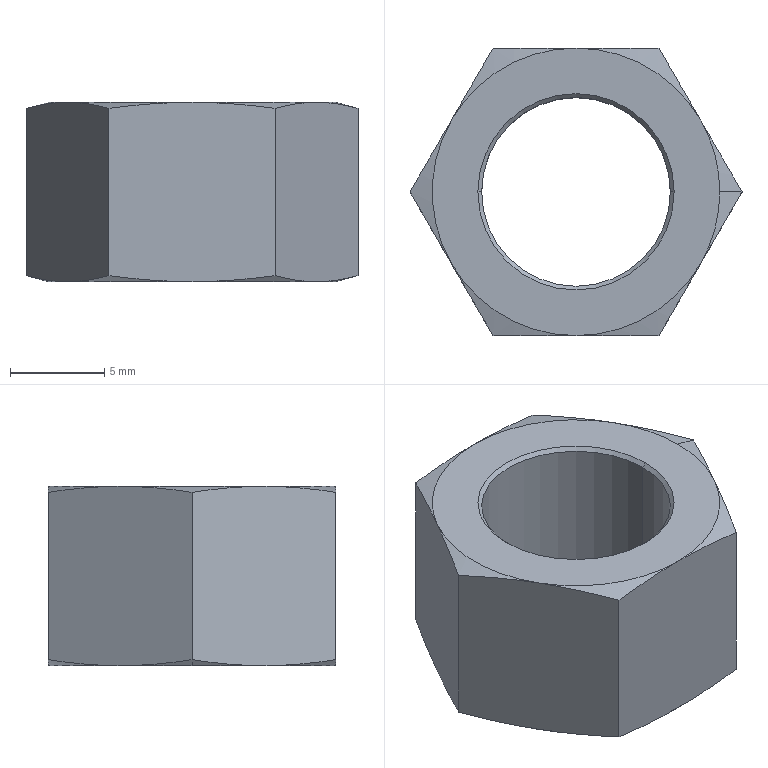Part | SolidWorks | features Cut 2, Chamfer 1, Extrusion 1 | 1 solid | 28 faces | box 17.59 x 15.233 x 9.5 mm | volume 1158 mm3 | cone 18 | plane 8 | cylinder 2 | commonest cylinder face diameters 10 x2
STEP:
#1=CARTESIAN_POINT('',(-5.,0.,9.3));
#2=VERTEX_POINT('',#1);
#3=CARTESIAN_POINT('',(5.,0.,9.3));
#4=VERTEX_POINT('',#3);
#5=CARTESIAN_POINT('',(0.,0.,9.3));
#6=DIRECTION('',(0.,0.,1.));
#7=DIRECTION('',(1.,0.,0.));
#8=AXIS2_PLACEMENT_3D('',#5,#6,#7);
#9=CIRCLE('',#8,5.);
#10=EDGE_CURVE('',#2,#4,#9,.T.);
#11=ORIENTED_EDGE('',*,*,#10,.F.);
#12=CARTESIAN_POINT('',(-5.2,0.,9.5));
#13=VERTEX_POINT('',#12);
#14=CARTESIAN_POINT('',(-5.,0.,9.3));
#15=DIRECTION('',(-0.7071,0.,0.7071));
#16=VECTOR('',#15,1000.);
#17=LINE('',#14,#16);
#18=EDGE_CURVE('',#2,#13,#17,.T.);
#19=ORIENTED_EDGE('',*,*,#18,.T.);
#20=CARTESIAN_POINT('',(5.2,0.,9.5));
#21=VERTEX_POINT('',#20);
#22=CARTESIAN_POINT('',(0.,0.,9.5));
#23=DIRECTION('',(0.,0.,-1.));
#24=DIRECTION('',(1.,0.,0.));
#25=AXIS2_PLACEMENT_3D('',#22,#23,#24);
#26=CIRCLE('',#25,5.2);
#27=EDGE_CURVE('',#21,#13,#26,.T.);
#28=ORIENTED_EDGE('',*,*,#27,.F.);
#29=CARTESIAN_POINT('',(5.,0.,9.3));
#30=DIRECTION('',(0.7071,0.,0.7071));
#31=VECTOR('',#30,1000.);
#32=LINE('',#29,#31);
#33=EDGE_CURVE('',#4,#21,#32,.T.);
#34=ORIENTED_EDGE('',*,*,#33,.F.);
#35=EDGE_LOOP('',(#11,#19,#28,#34));
#36=FACE_OUTER_BOUND('',#35,.T.);
#37=CARTESIAN_POINT('',(0.,0.,9.3));
#38=DIRECTION('',(0.,0.,1.));
#39=DIRECTION('',(1.,0.,0.));
#40=AXIS2_PLACEMENT_3D('',#37,#38,#39);
#41=CONICAL_SURFACE('',#40,5.,0.7854);
#42=ADVANCED_FACE('',(#36),#41,.F.);
#43=CARTESIAN_POINT('',(5.,0.,0.2));
#44=VERTEX_POINT('',#43);
#45=CARTESIAN_POINT('',(-5.,0.,0.2));
#46=VERTEX_POINT('',#45);
#47=CARTESIAN_POINT('',(0.,0.,0.2));
#48=DIRECTION('',(0.,0.,-1.));
#49=DIRECTION('',(1.,0.,0.));
#50=AXIS2_PLACEMENT_3D('',#47,#48,#49);
#51=CIRCLE('',#50,5.);
#52=EDGE_CURVE('',#44,#46,#51,.T.);
#53=ORIENTED_EDGE('',*,*,#52,.F.);
#54=CARTESIAN_POINT('',(5.2,0.,0.));
#55=VERTEX_POINT('',#54);
#56=CARTESIAN_POINT('',(5.2,0.,0.));
#57=DIRECTION('',(0.7071,0.,-0.7071));
#58=VECTOR('',#57,1000.);
#59=LINE('',#56,#58);
#60=EDGE_CURVE('',#44,#55,#59,.T.);
#61=ORIENTED_EDGE('',*,*,#60,.T.);
#62=CARTESIAN_POINT('',(-5.2,0.,0.));
#63=VERTEX_POINT('',#62);
#64=CARTESIAN_POINT('',(0.,0.,0.));
#65=DIRECTION('',(0.,0.,1.));
#66=DIRECTION('',(1.,0.,0.));
#67=AXIS2_PLACEMENT_3D('',#64,#65,#66);
#68=CIRCLE('',#67,5.2);
#69=EDGE_CURVE('',#63,#55,#68,.T.);
#70=ORIENTED_EDGE('',*,*,#69,.F.);
#71=CARTESIAN_POINT('',(-5.2,0.,0.));
#72=DIRECTION('',(-0.7071,0.,-0.7071));
#73=VECTOR('',#72,1000.);
#74=LINE('',#71,#73);
#75=EDGE_CURVE('',#46,#63,#74,.T.);
#76=ORIENTED_EDGE('',*,*,#75,.F.);
#77=EDGE_LOOP('',(#53,#61,#70,#76));
#78=FACE_OUTER_BOUND('',#77,.T.);
#79=CARTESIAN_POINT('',(0.,0.,0.));
#80=DIRECTION('',(0.,0.,-1.));
#81=DIRECTION('',(-1.,0.,0.));
#82=AXIS2_PLACEMENT_3D('',#79,#80,#81);
#83=CONICAL_SURFACE('',#82,5.2,0.7854);
#84=ADVANCED_FACE('',(#78),#83,.F.);
#85=CARTESIAN_POINT('',(7.617,0.,9.5));
#86=VERTEX_POINT('',#85);
#87=CARTESIAN_POINT('',(6.596,3.808,9.5));
#88=VERTEX_POINT('',#87);
#89=CARTESIAN_POINT('',(0.,0.,9.5));
#90=DIRECTION('',(0.,0.,1.));
#91=DIRECTION('',(1.,0.,0.));
#92=AXIS2_PLACEMENT_3D('',#89,#90,#91);
#93=CIRCLE('',#92,7.617);
#94=EDGE_CURVE('',#86,#88,#93,.T.);
#95=ORIENTED_EDGE('',*,*,#94,.F.);
#96=CARTESIAN_POINT('',(8.795,0.,9.184));
#97=VERTEX_POINT('',#96);
#98=CARTESIAN_POINT('',(7.617,0.,9.5));
#99=DIRECTION('',(0.9659,0.,-0.2588));
#100=VECTOR('',#99,1000.);
#101=LINE('',#98,#100);
#102=EDGE_CURVE('',#86,#97,#101,.T.);
#103=ORIENTED_EDGE('',*,*,#102,.T.);
#104=CARTESIAN_POINT('',(8.795,0.,9.184));
#105=CARTESIAN_POINT('',(8.062,1.269,9.381));
#106=CARTESIAN_POINT('',(7.329,2.539,9.5));
#107=CARTESIAN_POINT('',(6.596,3.808,9.5));
#108=B_SPLINE_CURVE_WITH_KNOTS('',3,(#104,#105,#106,#107),.UNSPECIFIED.,.F.,.F.,(4,4),(0.000000231,0.004398),.UNSPECIFIED.);
#109=EDGE_CURVE('',#97,#88,#108,.T.);
#110=ORIENTED_EDGE('',*,*,#109,.T.);
#111=EDGE_LOOP('',(#95,#103,#110));
#112=FACE_OUTER_BOUND('',#111,.T.);
#113=CARTESIAN_POINT('',(0.,0.,9.5));
#114=DIRECTION('',(0.,0.,-1.));
#115=DIRECTION('',(1.,0.,0.));
#116=AXIS2_PLACEMENT_3D('',#113,#114,#115);
#117=CONICAL_SURFACE('',#116,7.617,1.309);
#118=ADVANCED_FACE('',(#112),#117,.T.);
#119=CARTESIAN_POINT('',(-7.617,0.,0.));
#120=VERTEX_POINT('',#119);
#121=CARTESIAN_POINT('',(-6.596,3.808,0.));
#122=VERTEX_POINT('',#121);
#123=CARTESIAN_POINT('',(0.,0.,0.));
#124=DIRECTION('',(0.,0.,-1.));
#125=DIRECTION('',(-1.,0.,0.));
#126=AXIS2_PLACEMENT_3D('',#123,#124,#125);
#127=CIRCLE('',#126,7.617);
#128=EDGE_CURVE('',#120,#122,#127,.T.);
#129=ORIENTED_EDGE('',*,*,#128,.F.);
#130=CARTESIAN_POINT('',(-8.795,0.,0.3157));
#131=VERTEX_POINT('',#130);
#132=CARTESIAN_POINT('',(-7.617,0.,0.));
#133=DIRECTION('',(-0.9659,0.,0.2588));
#134=VECTOR('',#133,1000.);
#135=LINE('',#132,#134);
#136=EDGE_CURVE('',#120,#131,#135,.T.);
#137=ORIENTED_EDGE('',*,*,#136,.T.);
#138=CARTESIAN_POINT('',(-8.795,0.,0.3157));
#139=CARTESIAN_POINT('',(-8.062,1.269,0.1193));
#140=CARTESIAN_POINT('',(-7.329,2.539,0.));
#141=CARTESIAN_POINT('',(-6.596,3.808,0.));
#142=B_SPLINE_CURVE_WITH_KNOTS('',3,(#138,#139,#140,#141),.UNSPECIFIED.,.F.,.F.,(4,4),(0.000000231,0.004398),.UNSPECIFIED.);
#143=EDGE_CURVE('',#131,#122,#142,.T.);
#144=ORIENTED_EDGE('',*,*,#143,.T.);
#145=EDGE_LOOP('',(#129,#137,#144));
#146=FACE_OUTER_BOUND('',#145,.T.);
#147=CARTESIAN_POINT('',(0.,0.,0.));
#148=DIRECTION('',(0.,0.,1.));
#149=DIRECTION('',(-1.,0.,0.));
#150=AXIS2_PLACEMENT_3D('',#147,#148,#149);
#151=CONICAL_SURFACE('',#150,7.617,1.309);
#152=ADVANCED_FACE('',(#146),#151,.T.);
#153=ORIENTED_EDGE('',*,*,#10,.T.);
#154=CARTESIAN_POINT('',(5.,0.,9.5));
#155=DIRECTION('',(0.,0.,-1.));
#156=VECTOR('',#155,1000.);
#157=LINE('',#154,#156);
#158=EDGE_CURVE('',#4,#44,#157,.T.);
#159=ORIENTED_EDGE('',*,*,#158,.T.);
#160=ORIENTED_EDGE('',*,*,#52,.T.);
#161=CARTESIAN_POINT('',(-5.,0.,9.5));
#162=DIRECTION('',(0.,0.,-1.));
#163=VECTOR('',#162,1000.);
#164=LINE('',#161,#163);
#165=EDGE_CURVE('',#2,#46,#164,.T.);
#166=ORIENTED_EDGE('',*,*,#165,.F.);
#167=EDGE_LOOP('',(#153,#159,#160,#166));
#168=FACE_OUTER_BOUND('',#167,.T.);
#169=CARTESIAN_POINT('',(0.,0.,9.5));
#170=DIRECTION('',(0.,0.,-1.));
#171=DIRECTION('',(-1.,0.,0.));
#172=AXIS2_PLACEMENT_3D('',#169,#170,#171);
#173=CYLINDRICAL_SURFACE('',#172,5.);
#174=ADVANCED_FACE('',(#168),#173,.F.);
#175=ORIENTED_EDGE('',*,*,#109,.F.);
#176=CARTESIAN_POINT('',(8.795,0.,0.3157));
#177=VERTEX_POINT('',#176);
#178=CARTESIAN_POINT('',(8.795,0.,9.5));
#179=DIRECTION('',(0.,0.,-1.));
#180=VECTOR('',#179,1000.);
#181=LINE('',#178,#180);
#182=EDGE_CURVE('',#97,#177,#181,.T.);
#183=ORIENTED_EDGE('',*,*,#182,.T.);
#184=CARTESIAN_POINT('',(6.596,3.808,0.));
#185=VERTEX_POINT('',#184);
#186=CARTESIAN_POINT('',(6.596,3.808,0.));
#187=CARTESIAN_POINT('',(7.329,2.539,0.));
#188=CARTESIAN_POINT('',(8.062,1.269,0.1193));
#189=CARTESIAN_POINT('',(8.795,0.,0.3157));
#190=B_SPLINE_CURVE_WITH_KNOTS('',3,(#186,#187,#188,#189),.UNSPECIFIED.,.F.,.F.,(4,4),(0.004398,0.008795),.UNSPECIFIED.);
#191=EDGE_CURVE('',#185,#177,#190,.T.);
#192=ORIENTED_EDGE('',*,*,#191,.F.);
#193=CARTESIAN_POINT('',(4.398,7.617,0.3157));
#194=VERTEX_POINT('',#193);
#195=CARTESIAN_POINT('',(4.398,7.617,0.3157));
#196=CARTESIAN_POINT('',(5.13,6.347,0.1193));
#197=CARTESIAN_POINT('',(5.863,5.078,0.));
#198=CARTESIAN_POINT('',(6.596,3.808,0.));
#199=B_SPLINE_CURVE_WITH_KNOTS('',3,(#195,#196,#197,#198),.UNSPECIFIED.,.F.,.F.,(4,4),(0.000000231,0.004398),.UNSPECIFIED.);
#200=EDGE_CURVE('',#194,#185,#199,.T.);
#201=ORIENTED_EDGE('',*,*,#200,.F.);
#202=CARTESIAN_POINT('',(4.398,7.617,9.184));
#203=VERTEX_POINT('',#202);
#204=CARTESIAN_POINT('',(4.398,7.617,9.5));
#205=DIRECTION('',(0.,0.,-1.));
#206=VECTOR('',#205,1000.);
#207=LINE('',#204,#206);
#208=EDGE_CURVE('',#203,#194,#207,.T.);
#209=ORIENTED_EDGE('',*,*,#208,.F.);
#210=CARTESIAN_POINT('',(6.596,3.808,9.5));
#211=CARTESIAN_POINT('',(5.863,5.078,9.5));
#212=CARTESIAN_POINT('',(5.13,6.347,9.381));
#213=CARTESIAN_POINT('',(4.398,7.617,9.184));
#214=B_SPLINE_CURVE_WITH_KNOTS('',3,(#210,#211,#212,#213),.UNSPECIFIED.,.F.,.F.,(4,4),(0.004398,0.008795),.UNSPECIFIED.);
#215=EDGE_CURVE('',#88,#203,#214,.T.);
#216=ORIENTED_EDGE('',*,*,#215,.F.);
#217=EDGE_LOOP('',(#175,#183,#192,#201,#209,#216));
#218=FACE_OUTER_BOUND('',#217,.T.);
#219=CARTESIAN_POINT('',(8.795,0.,9.5));
#220=DIRECTION('',(-0.866,-0.5,0.));
#221=DIRECTION('',(0.5,-0.866,0.));
#222=AXIS2_PLACEMENT_3D('',#219,#220,#221);
#223=PLANE('',#222);
#224=ADVANCED_FACE('',(#218),#223,.F.);
#225=CARTESIAN_POINT('',(0.,7.617,9.5));
#226=VERTEX_POINT('',#225);
#227=CARTESIAN_POINT('',(4.398,7.617,9.184));
#228=CARTESIAN_POINT('',(2.934,7.617,9.38));
#229=CARTESIAN_POINT('',(1.469,7.617,9.5));
#230=CARTESIAN_POINT('',(0.,7.617,9.5));
#231=B_SPLINE_CURVE_WITH_KNOTS('',3,(#227,#228,#229,#230),.UNSPECIFIED.,.F.,.F.,(4,4),(0.02453,0.02896),.UNSPECIFIED.);
#232=EDGE_CURVE('',#203,#226,#231,.T.);
#233=ORIENTED_EDGE('',*,*,#232,.F.);
#234=ORIENTED_EDGE('',*,*,#208,.T.);
#235=CARTESIAN_POINT('',(0.,7.617,0.));
#236=VERTEX_POINT('',#235);
#237=CARTESIAN_POINT('',(0.,7.617,0.));
#238=CARTESIAN_POINT('',(1.469,7.617,0.));
#239=CARTESIAN_POINT('',(2.934,7.617,0.1197));
#240=CARTESIAN_POINT('',(4.398,7.617,0.3157));
#241=B_SPLINE_CURVE_WITH_KNOTS('',3,(#237,#238,#239,#240),.UNSPECIFIED.,.F.,.F.,(4,4),(0.01193,0.01636),.UNSPECIFIED.);
#242=EDGE_CURVE('',#236,#194,#241,.T.);
#243=ORIENTED_EDGE('',*,*,#242,.F.);
#244=CARTESIAN_POINT('',(-4.397,7.617,0.3157));
#245=VERTEX_POINT('',#244);
#246=CARTESIAN_POINT('',(-4.397,7.617,0.3157));
#247=CARTESIAN_POINT('',(-3.667,7.617,0.2178));
#248=CARTESIAN_POINT('',(-2.931,7.617,0.1378));
#249=CARTESIAN_POINT('',(-1.465,7.617,0.0288));
#250=CARTESIAN_POINT('',(-0.7319,7.617,0.));
#251=CARTESIAN_POINT('',(0.,7.617,0.));
#252=B_SPLINE_CURVE_WITH_KNOTS('',3,(#246,#247,#248,#249,#250,#251),.UNSPECIFIED.,.F.,.F.,(4,2,4),(0.007509,0.009719,0.01193),.UNSPECIFIED.);
#253=EDGE_CURVE('',#245,#236,#252,.T.);
#254=ORIENTED_EDGE('',*,*,#253,.F.);
#255=CARTESIAN_POINT('',(-4.397,7.617,9.184));
#256=VERTEX_POINT('',#255);
#257=CARTESIAN_POINT('',(-4.397,7.617,9.5));
#258=DIRECTION('',(0.,0.,-1.));
#259=VECTOR('',#258,1000.);
#260=LINE('',#257,#259);
#261=EDGE_CURVE('',#256,#245,#260,.T.);
#262=ORIENTED_EDGE('',*,*,#261,.F.);
#263=CARTESIAN_POINT('',(0.,7.617,9.5));
#264=CARTESIAN_POINT('',(-0.7319,7.617,9.5));
#265=CARTESIAN_POINT('',(-1.465,7.617,9.471));
#266=CARTESIAN_POINT('',(-2.931,7.617,9.362));
#267=CARTESIAN_POINT('',(-3.667,7.617,9.282));
#268=CARTESIAN_POINT('',(-4.397,7.617,9.184));
#269=B_SPLINE_CURVE_WITH_KNOTS('',3,(#263,#264,#265,#266,#267,#268),.UNSPECIFIED.,.F.,.F.,(4,2,4),(0.02896,0.03116,0.03337),.UNSPECIFIED.);
#270=EDGE_CURVE('',#226,#256,#269,.T.);
#271=ORIENTED_EDGE('',*,*,#270,.F.);
#272=EDGE_LOOP('',(#233,#234,#243,#254,#262,#271));
#273=FACE_OUTER_BOUND('',#272,.T.);
#274=CARTESIAN_POINT('',(4.398,7.617,9.5));
#275=DIRECTION('',(0.,-1.,0.));
#276=DIRECTION('',(0.,0.,-1.));
#277=AXIS2_PLACEMENT_3D('',#274,#275,#276);
#278=PLANE('',#277);
#279=ADVANCED_FACE('',(#273),#278,.F.);
#280=CARTESIAN_POINT('',(-6.596,3.808,9.5));
#281=VERTEX_POINT('',#280);
#282=CARTESIAN_POINT('',(-4.397,7.617,9.184));
#283=CARTESIAN_POINT('',(-5.13,6.347,9.381));
#284=CARTESIAN_POINT('',(-5.863,5.078,9.5));
#285=CARTESIAN_POINT('',(-6.596,3.808,9.5));
#286=B_SPLINE_CURVE_WITH_KNOTS('',3,(#282,#283,#284,#285),.UNSPECIFIED.,.F.,.F.,(4,4),(0.000000231,0.004398),.UNSPECIFIED.);
#287=EDGE_CURVE('',#256,#281,#286,.T.);
#288=ORIENTED_EDGE('',*,*,#287,.F.);
#289=ORIENTED_EDGE('',*,*,#261,.T.);
#290=CARTESIAN_POINT('',(-6.596,3.808,0.));
#291=CARTESIAN_POINT('',(-5.863,5.078,0.));
#292=CARTESIAN_POINT('',(-5.13,6.347,0.1193));
#293=CARTESIAN_POINT('',(-4.397,7.617,0.3157));
#294=B_SPLINE_CURVE_WITH_KNOTS('',3,(#290,#291,#292,#293),.UNSPECIFIED.,.F.,.F.,(4,4),(0.004398,0.008795),.UNSPECIFIED.);
#295=EDGE_CURVE('',#122,#245,#294,.T.);
#296=ORIENTED_EDGE('',*,*,#295,.F.);
#297=ORIENTED_EDGE('',*,*,#143,.F.);
#298=CARTESIAN_POINT('',(-8.795,0.,9.184));
#299=VERTEX_POINT('',#298);
#300=CARTESIAN_POINT('',(-8.795,0.,9.5));
#301=DIRECTION('',(0.,0.,-1.));
#302=VECTOR('',#301,1000.);
#303=LINE('',#300,#302);
#304=EDGE_CURVE('',#299,#131,#303,.T.);
#305=ORIENTED_EDGE('',*,*,#304,.F.);
#306=CARTESIAN_POINT('',(-6.596,3.808,9.5));
#307=CARTESIAN_POINT('',(-7.329,2.539,9.5));
#308=CARTESIAN_POINT('',(-8.062,1.269,9.381));
#309=CARTESIAN_POINT('',(-8.795,0.,9.184));
#310=B_SPLINE_CURVE_WITH_KNOTS('',3,(#306,#307,#308,#309),.UNSPECIFIED.,.F.,.F.,(4,4),(0.004398,0.008795),.UNSPECIFIED.);
#311=EDGE_CURVE('',#281,#299,#310,.T.);
#312=ORIENTED_EDGE('',*,*,#311,.F.);
#313=EDGE_LOOP('',(#288,#289,#296,#297,#305,#312));
#314=FACE_OUTER_BOUND('',#313,.T.);
#315=CARTESIAN_POINT('',(-4.397,7.617,9.5));
#316=DIRECTION('',(0.866,-0.5,0.));
#317=DIRECTION('',(0.5,0.866,0.));
#318=AXIS2_PLACEMENT_3D('',#315,#316,#317);
#319=PLANE('',#318);
#320=ADVANCED_FACE('',(#314),#319,.F.);
#321=CARTESIAN_POINT('',(-6.596,-3.808,9.5));
#322=VERTEX_POINT('',#321);
#323=CARTESIAN_POINT('',(-8.795,0.,9.184));
#324=CARTESIAN_POINT('',(-8.062,-1.269,9.381));
#325=CARTESIAN_POINT('',(-7.329,-2.539,9.5));
#326=CARTESIAN_POINT('',(-6.596,-3.808,9.5));
#327=B_SPLINE_CURVE_WITH_KNOTS('',3,(#323,#324,#325,#326),.UNSPECIFIED.,.F.,.F.,(4,4),(0.000000231,0.004398),.UNSPECIFIED.);
#328=EDGE_CURVE('',#299,#322,#327,.T.);
#329=ORIENTED_EDGE('',*,*,#328,.F.);
#330=ORIENTED_EDGE('',*,*,#304,.T.);
#331=CARTESIAN_POINT('',(-6.596,-3.808,0.));
#332=VERTEX_POINT('',#331);
#333=CARTESIAN_POINT('',(-6.596,-3.808,0.));
#334=CARTESIAN_POINT('',(-7.329,-2.539,0.));
#335=CARTESIAN_POINT('',(-8.062,-1.269,0.1193));
#336=CARTESIAN_POINT('',(-8.795,0.,0.3157));
#337=B_SPLINE_CURVE_WITH_KNOTS('',3,(#333,#334,#335,#336),.UNSPECIFIED.,.F.,.F.,(4,4),(0.004398,0.008795),.UNSPECIFIED.);
#338=EDGE_CURVE('',#332,#131,#337,.T.);
#339=ORIENTED_EDGE('',*,*,#338,.F.);
#340=CARTESIAN_POINT('',(-4.397,-7.617,0.3157));
#341=VERTEX_POINT('',#340);
#342=CARTESIAN_POINT('',(-4.397,-7.617,0.3157));
#343=CARTESIAN_POINT('',(-5.13,-6.347,0.1193));
#344=CARTESIAN_POINT('',(-5.863,-5.078,0.));
#345=CARTESIAN_POINT('',(-6.596,-3.808,0.));
#346=B_SPLINE_CURVE_WITH_KNOTS('',3,(#342,#343,#344,#345),.UNSPECIFIED.,.F.,.F.,(4,4),(0.000000231,0.004398),.UNSPECIFIED.);
#347=EDGE_CURVE('',#341,#332,#346,.T.);
#348=ORIENTED_EDGE('',*,*,#347,.F.);
#349=CARTESIAN_POINT('',(-4.397,-7.617,9.184));
#350=VERTEX_POINT('',#349);
#351=CARTESIAN_POINT('',(-4.397,-7.617,9.5));
#352=DIRECTION('',(0.,0.,-1.));
#353=VECTOR('',#352,1000.);
#354=LINE('',#351,#353);
#355=EDGE_CURVE('',#350,#341,#354,.T.);
#356=ORIENTED_EDGE('',*,*,#355,.F.);
#357=CARTESIAN_POINT('',(-6.596,-3.808,9.5));
#358=CARTESIAN_POINT('',(-5.863,-5.078,9.5));
#359=CARTESIAN_POINT('',(-5.13,-6.347,9.381));
#360=CARTESIAN_POINT('',(-4.397,-7.617,9.184));
#361=B_SPLINE_CURVE_WITH_KNOTS('',3,(#357,#358,#359,#360),.UNSPECIFIED.,.F.,.F.,(4,4),(0.004398,0.008795),.UNSPECIFIED.);
#362=EDGE_CURVE('',#322,#350,#361,.T.);
#363=ORIENTED_EDGE('',*,*,#362,.F.);
#364=EDGE_LOOP('',(#329,#330,#339,#348,#356,#363));
#365=FACE_OUTER_BOUND('',#364,.T.);
#366=CARTESIAN_POINT('',(-8.795,0.,9.5));
#367=DIRECTION('',(0.866,0.5,0.));
#368=DIRECTION('',(-0.5,0.866,0.));
#369=AXIS2_PLACEMENT_3D('',#366,#367,#368);
#370=PLANE('',#369);
#371=ADVANCED_FACE('',(#365),#370,.F.);
#372=CARTESIAN_POINT('',(0.,-7.617,9.5));
#373=VERTEX_POINT('',#372);
#374=CARTESIAN_POINT('',(-4.397,-7.617,9.184));
#375=CARTESIAN_POINT('',(-3.667,-7.617,9.282));
#376=CARTESIAN_POINT('',(-2.931,-7.617,9.362));
#377=CARTESIAN_POINT('',(-1.465,-7.617,9.471));
#378=CARTESIAN_POINT('',(-0.7319,-7.617,9.5));
#379=CARTESIAN_POINT('',(0.,-7.617,9.5));
#380=B_SPLINE_CURVE_WITH_KNOTS('',3,(#374,#375,#376,#377,#378,#379),.UNSPECIFIED.,.F.,.F.,(4,2,4),(0.007509,0.009719,0.01193),.UNSPECIFIED.);
#381=EDGE_CURVE('',#350,#373,#380,.T.);
#382=ORIENTED_EDGE('',*,*,#381,.F.);
#383=ORIENTED_EDGE('',*,*,#355,.T.);
#384=CARTESIAN_POINT('',(0.,-7.617,0.));
#385=VERTEX_POINT('',#384);
#386=CARTESIAN_POINT('',(0.,-7.617,0.));
#387=CARTESIAN_POINT('',(-0.7319,-7.617,0.));
#388=CARTESIAN_POINT('',(-1.465,-7.617,0.0288));
#389=CARTESIAN_POINT('',(-2.931,-7.617,0.1378));
#390=CARTESIAN_POINT('',(-3.667,-7.617,0.2178));
#391=CARTESIAN_POINT('',(-4.397,-7.617,0.3157));
#392=B_SPLINE_CURVE_WITH_KNOTS('',3,(#386,#387,#388,#389,#390,#391),.UNSPECIFIED.,.F.,.F.,(4,2,4),(0.02896,0.03116,0.03337),.UNSPECIFIED.);
#393=EDGE_CURVE('',#385,#341,#392,.T.);
#394=ORIENTED_EDGE('',*,*,#393,.F.);
#395=CARTESIAN_POINT('',(4.398,-7.617,0.3157));
#396=VERTEX_POINT('',#395);
#397=CARTESIAN_POINT('',(4.398,-7.617,0.3157));
#398=CARTESIAN_POINT('',(2.934,-7.617,0.1197));
#399=CARTESIAN_POINT('',(1.469,-7.617,0.));
#400=CARTESIAN_POINT('',(0.,-7.617,0.));
#401=B_SPLINE_CURVE_WITH_KNOTS('',3,(#397,#398,#399,#400),.UNSPECIFIED.,.F.,.F.,(4,4),(0.02453,0.02896),.UNSPECIFIED.);
#402=EDGE_CURVE('',#396,#385,#401,.T.);
#403=ORIENTED_EDGE('',*,*,#402,.F.);
#404=CARTESIAN_POINT('',(4.398,-7.617,9.184));
#405=VERTEX_POINT('',#404);
#406=CARTESIAN_POINT('',(4.398,-7.617,9.5));
#407=DIRECTION('',(0.,0.,-1.));
#408=VECTOR('',#407,1000.);
#409=LINE('',#406,#408);
#410=EDGE_CURVE('',#405,#396,#409,.T.);
#411=ORIENTED_EDGE('',*,*,#410,.F.);
#412=CARTESIAN_POINT('',(0.,-7.617,9.5));
#413=CARTESIAN_POINT('',(1.469,-7.617,9.5));
#414=CARTESIAN_POINT('',(2.934,-7.617,9.38));
#415=CARTESIAN_POINT('',(4.398,-7.617,9.184));
#416=B_SPLINE_CURVE_WITH_KNOTS('',3,(#412,#413,#414,#415),.UNSPECIFIED.,.F.,.F.,(4,4),(0.01193,0.01636),.UNSPECIFIED.);
#417=EDGE_CURVE('',#373,#405,#416,.T.);
#418=ORIENTED_EDGE('',*,*,#417,.F.);
#419=EDGE_LOOP('',(#382,#383,#394,#403,#411,#418));
#420=FACE_OUTER_BOUND('',#419,.T.);
#421=CARTESIAN_POINT('',(-4.397,-7.617,9.5));
#422=DIRECTION('',(0.,1.,0.));
#423=DIRECTION('',(0.,0.,1.));
#424=AXIS2_PLACEMENT_3D('',#421,#422,#423);
#425=PLANE('',#424);
#426=ADVANCED_FACE('',(#420),#425,.F.);
#427=CARTESIAN_POINT('',(6.596,-3.808,9.5));
#428=VERTEX_POINT('',#427);
#429=CARTESIAN_POINT('',(4.398,-7.617,9.184));
#430=CARTESIAN_POINT('',(5.13,-6.347,9.381));
#431=CARTESIAN_POINT('',(5.863,-5.078,9.5));
#432=CARTESIAN_POINT('',(6.596,-3.808,9.5));
#433=B_SPLINE_CURVE_WITH_KNOTS('',3,(#429,#430,#431,#432),.UNSPECIFIED.,.F.,.F.,(4,4),(0.000000231,0.004398),.UNSPECIFIED.);
#434=EDGE_CURVE('',#405,#428,#433,.T.);
#435=ORIENTED_EDGE('',*,*,#434,.F.);
#436=ORIENTED_EDGE('',*,*,#410,.T.);
#437=CARTESIAN_POINT('',(6.596,-3.808,0.));
#438=VERTEX_POINT('',#437);
#439=CARTESIAN_POINT('',(6.596,-3.808,0.));
#440=CARTESIAN_POINT('',(5.863,-5.078,0.));
#441=CARTESIAN_POINT('',(5.13,-6.347,0.1193));
#442=CARTESIAN_POINT('',(4.398,-7.617,0.3157));
#443=B_SPLINE_CURVE_WITH_KNOTS('',3,(#439,#440,#441,#442),.UNSPECIFIED.,.F.,.F.,(4,4),(0.004398,0.008795),.UNSPECIFIED.);
#444=EDGE_CURVE('',#438,#396,#443,.T.);
#445=ORIENTED_EDGE('',*,*,#444,.F.);
#446=CARTESIAN_POINT('',(8.795,0.,0.3157));
#447=CARTESIAN_POINT('',(8.062,-1.269,0.1193));
#448=CARTESIAN_POINT('',(7.329,-2.539,0.));
#449=CARTESIAN_POINT('',(6.596,-3.808,0.));
#450=B_SPLINE_CURVE_WITH_KNOTS('',3,(#446,#447,#448,#449),.UNSPECIFIED.,.F.,.F.,(4,4),(0.000000231,0.004398),.UNSPECIFIED.);
#451=EDGE_CURVE('',#177,#438,#450,.T.);
#452=ORIENTED_EDGE('',*,*,#451,.F.);
#453=ORIENTED_EDGE('',*,*,#182,.F.);
#454=CARTESIAN_POINT('',(6.596,-3.808,9.5));
#455=CARTESIAN_POINT('',(7.329,-2.539,9.5));
#456=CARTESIAN_POINT('',(8.062,-1.269,9.381));
#457=CARTESIAN_POINT('',(8.795,0.,9.184));
#458=B_SPLINE_CURVE_WITH_KNOTS('',3,(#454,#455,#456,#457),.UNSPECIFIED.,.F.,.F.,(4,4),(0.004398,0.008795),.UNSPECIFIED.);
#459=EDGE_CURVE('',#428,#97,#458,.T.);
#460=ORIENTED_EDGE('',*,*,#459,.F.);
#461=EDGE_LOOP('',(#435,#436,#445,#452,#453,#460));
#462=FACE_OUTER_BOUND('',#461,.T.);
#463=CARTESIAN_POINT('',(4.398,-7.617,9.5));
#464=DIRECTION('',(-0.866,0.5,0.));
#465=DIRECTION('',(-0.5,-0.866,0.));
#466=AXIS2_PLACEMENT_3D('',#463,#464,#465);
#467=PLANE('',#466);
#468=ADVANCED_FACE('',(#462),#467,.F.);
#469=ORIENTED_EDGE('',*,*,#27,.T.);
#470=CARTESIAN_POINT('',(0.,0.,9.5));
#471=DIRECTION('',(0.,0.,-1.));
#472=DIRECTION('',(1.,0.,0.));
#473=AXIS2_PLACEMENT_3D('',#470,#471,#472);
#474=CIRCLE('',#473,5.2);
#475=EDGE_CURVE('',#13,#21,#474,.T.);
#476=ORIENTED_EDGE('',*,*,#475,.T.);
#477=EDGE_LOOP('',(#469,#476));
#478=FACE_BOUND('',#477,.T.);
#479=CARTESIAN_POINT('',(0.,0.,9.5));
#480=DIRECTION('',(0.,0.,1.));
#481=DIRECTION('',(1.,0.,0.));
#482=AXIS2_PLACEMENT_3D('',#479,#480,#481);
#483=CIRCLE('',#482,7.617);
#484=EDGE_CURVE('',#428,#86,#483,.T.);
#485=ORIENTED_EDGE('',*,*,#484,.T.);
#486=ORIENTED_EDGE('',*,*,#94,.T.);
#487=CARTESIAN_POINT('',(0.,0.,9.5));
#488=DIRECTION('',(0.,0.,1.));
#489=DIRECTION('',(1.,0.,0.));
#490=AXIS2_PLACEMENT_3D('',#487,#488,#489);
#491=CIRCLE('',#490,7.617);
#492=EDGE_CURVE('',#88,#226,#491,.T.);
#493=ORIENTED_EDGE('',*,*,#492,.T.);
#494=CARTESIAN_POINT('',(0.,0.,9.5));
#495=DIRECTION('',(0.,0.,1.));
#496=DIRECTION('',(1.,0.,0.));
#497=AXIS2_PLACEMENT_3D('',#494,#495,#496);
#498=CIRCLE('',#497,7.617);
#499=EDGE_CURVE('',#226,#281,#498,.T.);
#500=ORIENTED_EDGE('',*,*,#499,.T.);
#501=CARTESIAN_POINT('',(0.,0.,9.5));
#502=DIRECTION('',(0.,0.,1.));
#503=DIRECTION('',(1.,0.,0.));
#504=AXIS2_PLACEMENT_3D('',#501,#502,#503);
#505=CIRCLE('',#504,7.617);
#506=EDGE_CURVE('',#281,#322,#505,.T.);
#507=ORIENTED_EDGE('',*,*,#506,.T.);
#508=CARTESIAN_POINT('',(0.,0.,9.5));
#509=DIRECTION('',(0.,0.,1.));
#510=DIRECTION('',(1.,0.,0.));
#511=AXIS2_PLACEMENT_3D('',#508,#509,#510);
#512=CIRCLE('',#511,7.617);
#513=EDGE_CURVE('',#322,#373,#512,.T.);
#514=ORIENTED_EDGE('',*,*,#513,.T.);
#515=CARTESIAN_POINT('',(0.,0.,9.5));
#516=DIRECTION('',(0.,0.,1.));
#517=DIRECTION('',(1.,0.,0.));
#518=AXIS2_PLACEMENT_3D('',#515,#516,#517);
#519=CIRCLE('',#518,7.617);
#520=EDGE_CURVE('',#373,#428,#519,.T.);
#521=ORIENTED_EDGE('',*,*,#520,.T.);
#522=EDGE_LOOP('',(#485,#486,#493,#500,#507,#514,#521));
#523=FACE_OUTER_BOUND('',#522,.T.);
#524=CARTESIAN_POINT('',(4.398,7.617,9.5));
#525=DIRECTION('',(0.,0.,1.));
#526=DIRECTION('',(1.,0.,0.));
#527=AXIS2_PLACEMENT_3D('',#524,#525,#526);
#528=PLANE('',#527);
#529=ADVANCED_FACE('',(#478,#523),#528,.T.);
#530=ORIENTED_EDGE('',*,*,#69,.T.);
#531=CARTESIAN_POINT('',(0.,0.,0.));
#532=DIRECTION('',(0.,0.,1.));
#533=DIRECTION('',(1.,0.,0.));
#534=AXIS2_PLACEMENT_3D('',#531,#532,#533);
#535=CIRCLE('',#534,5.2);
#536=EDGE_CURVE('',#55,#63,#535,.T.);
#537=ORIENTED_EDGE('',*,*,#536,.T.);
#538=EDGE_LOOP('',(#530,#537));
#539=FACE_BOUND('',#538,.T.);
#540=CARTESIAN_POINT('',(0.,0.,0.));
#541=DIRECTION('',(0.,0.,-1.));
#542=DIRECTION('',(-1.,0.,0.));
#543=AXIS2_PLACEMENT_3D('',#540,#541,#542);
#544=CIRCLE('',#543,7.617);
#545=EDGE_CURVE('',#236,#185,#544,.T.);
#546=ORIENTED_EDGE('',*,*,#545,.T.);
#547=CARTESIAN_POINT('',(0.,0.,0.));
#548=DIRECTION('',(0.,0.,-1.));
#549=DIRECTION('',(-1.,0.,0.));
#550=AXIS2_PLACEMENT_3D('',#547,#548,#549);
#551=CIRCLE('',#550,7.617);
#552=EDGE_CURVE('',#185,#438,#551,.T.);
#553=ORIENTED_EDGE('',*,*,#552,.T.);
#554=CARTESIAN_POINT('',(0.,0.,0.));
#555=DIRECTION('',(0.,0.,-1.));
#556=DIRECTION('',(-1.,0.,0.));
#557=AXIS2_PLACEMENT_3D('',#554,#555,#556);
#558=CIRCLE('',#557,7.617);
#559=EDGE_CURVE('',#438,#385,#558,.T.);
#560=ORIENTED_EDGE('',*,*,#559,.T.);
#561=CARTESIAN_POINT('',(0.,0.,0.));
#562=DIRECTION('',(0.,0.,-1.));
#563=DIRECTION('',(-1.,0.,0.));
#564=AXIS2_PLACEMENT_3D('',#561,#562,#563);
#565=CIRCLE('',#564,7.617);
#566=EDGE_CURVE('',#385,#332,#565,.T.);
#567=ORIENTED_EDGE('',*,*,#566,.T.);
#568=CARTESIAN_POINT('',(0.,0.,0.));
#569=DIRECTION('',(0.,0.,-1.));
#570=DIRECTION('',(-1.,0.,0.));
#571=AXIS2_PLACEMENT_3D('',#568,#569,#570);
#572=CIRCLE('',#571,7.617);
#573=EDGE_CURVE('',#332,#120,#572,.T.);
#574=ORIENTED_EDGE('',*,*,#573,.T.);
#575=ORIENTED_EDGE('',*,*,#128,.T.);
#576=CARTESIAN_POINT('',(0.,0.,0.));
#577=DIRECTION('',(0.,0.,-1.));
#578=DIRECTION('',(-1.,0.,0.));
#579=AXIS2_PLACEMENT_3D('',#576,#577,#578);
#580=CIRCLE('',#579,7.617);
#581=EDGE_CURVE('',#122,#236,#580,.T.);
#582=ORIENTED_EDGE('',*,*,#581,.T.);
#583=EDGE_LOOP('',(#546,#553,#560,#567,#574,#575,#582));
#584=FACE_OUTER_BOUND('',#583,.T.);
#585=CARTESIAN_POINT('',(4.398,7.617,0.));
#586=DIRECTION('',(0.,0.,1.));
#587=DIRECTION('',(1.,0.,0.));
#588=AXIS2_PLACEMENT_3D('',#585,#586,#587);
#589=PLANE('',#588);
#590=ADVANCED_FACE('',(#539,#584),#589,.F.);
#591=ORIENTED_EDGE('',*,*,#158,.F.);
#592=CARTESIAN_POINT('',(0.,0.,9.3));
#593=DIRECTION('',(0.,0.,1.));
#594=DIRECTION('',(1.,0.,0.));
#595=AXIS2_PLACEMENT_3D('',#592,#593,#594);
#596=CIRCLE('',#595,5.);
#597=EDGE_CURVE('',#4,#2,#596,.T.);
#598=ORIENTED_EDGE('',*,*,#597,.T.);
#599=ORIENTED_EDGE('',*,*,#165,.T.);
#600=CARTESIAN_POINT('',(0.,0.,0.2));
#601=DIRECTION('',(0.,0.,-1.));
#602=DIRECTION('',(1.,0.,0.));
#603=AXIS2_PLACEMENT_3D('',#600,#601,#602);
#604=CIRCLE('',#603,5.);
#605=EDGE_CURVE('',#46,#44,#604,.T.);
#606=ORIENTED_EDGE('',*,*,#605,.T.);
#607=EDGE_LOOP('',(#591,#598,#599,#606));
#608=FACE_OUTER_BOUND('',#607,.T.);
#609=CARTESIAN_POINT('',(0.,0.,9.5));
#610=DIRECTION('',(0.,0.,-1.));
#611=DIRECTION('',(-1.,0.,0.));
#612=AXIS2_PLACEMENT_3D('',#609,#610,#611);
#613=CYLINDRICAL_SURFACE('',#612,5.);
#614=ADVANCED_FACE('',(#608),#613,.F.);
#615=ORIENTED_EDGE('',*,*,#402,.T.);
#616=ORIENTED_EDGE('',*,*,#559,.F.);
#617=ORIENTED_EDGE('',*,*,#444,.T.);
#618=EDGE_LOOP('',(#615,#616,#617));
#619=FACE_OUTER_BOUND('',#618,.T.);
#620=CARTESIAN_POINT('',(0.,0.,0.));
#621=DIRECTION('',(0.,0.,1.));
#622=DIRECTION('',(-1.,0.,0.));
#623=AXIS2_PLACEMENT_3D('',#620,#621,#622);
#624=CONICAL_SURFACE('',#623,7.617,1.309);
#625=ADVANCED_FACE('',(#619),#624,.T.);
#626=ORIENTED_EDGE('',*,*,#191,.T.);
#627=ORIENTED_EDGE('',*,*,#451,.T.);
#628=ORIENTED_EDGE('',*,*,#552,.F.);
#629=EDGE_LOOP('',(#626,#627,#628));
#630=FACE_OUTER_BOUND('',#629,.T.);
#631=CARTESIAN_POINT('',(0.,0.,0.));
#632=DIRECTION('',(0.,0.,1.));
#633=DIRECTION('',(-1.,0.,0.));
#634=AXIS2_PLACEMENT_3D('',#631,#632,#633);
#635=CONICAL_SURFACE('',#634,7.617,1.309);
#636=ADVANCED_FACE('',(#630),#635,.T.);
#637=ORIENTED_EDGE('',*,*,#347,.T.);
#638=ORIENTED_EDGE('',*,*,#566,.F.);
#639=ORIENTED_EDGE('',*,*,#393,.T.);
#640=EDGE_LOOP('',(#637,#638,#639));
#641=FACE_OUTER_BOUND('',#640,.T.);
#642=CARTESIAN_POINT('',(0.,0.,0.));
#643=DIRECTION('',(0.,0.,1.));
#644=DIRECTION('',(-1.,0.,0.));
#645=AXIS2_PLACEMENT_3D('',#642,#643,#644);
#646=CONICAL_SURFACE('',#645,7.617,1.309);
#647=ADVANCED_FACE('',(#641),#646,.T.);
#648=ORIENTED_EDGE('',*,*,#136,.F.);
#649=ORIENTED_EDGE('',*,*,#573,.F.);
#650=ORIENTED_EDGE('',*,*,#338,.T.);
#651=EDGE_LOOP('',(#648,#649,#650));
#652=FACE_OUTER_BOUND('',#651,.T.);
#653=CARTESIAN_POINT('',(0.,0.,0.));
#654=DIRECTION('',(0.,0.,1.));
#655=DIRECTION('',(-1.,0.,0.));
#656=AXIS2_PLACEMENT_3D('',#653,#654,#655);
#657=CONICAL_SURFACE('',#656,7.617,1.309);
#658=ADVANCED_FACE('',(#652),#657,.T.);
#659=ORIENTED_EDGE('',*,*,#295,.T.);
#660=ORIENTED_EDGE('',*,*,#253,.T.);
#661=ORIENTED_EDGE('',*,*,#581,.F.);
#662=EDGE_LOOP('',(#659,#660,#661));
#663=FACE_OUTER_BOUND('',#662,.T.);
#664=CARTESIAN_POINT('',(0.,0.,0.));
#665=DIRECTION('',(0.,0.,1.));
#666=DIRECTION('',(-1.,0.,0.));
#667=AXIS2_PLACEMENT_3D('',#664,#665,#666);
#668=CONICAL_SURFACE('',#667,7.617,1.309);
#669=ADVANCED_FACE('',(#663),#668,.T.);
#670=ORIENTED_EDGE('',*,*,#242,.T.);
#671=ORIENTED_EDGE('',*,*,#200,.T.);
#672=ORIENTED_EDGE('',*,*,#545,.F.);
#673=EDGE_LOOP('',(#670,#671,#672));
#674=FACE_OUTER_BOUND('',#673,.T.);
#675=CARTESIAN_POINT('',(0.,0.,0.));
#676=DIRECTION('',(0.,0.,1.));
#677=DIRECTION('',(-1.,0.,0.));
#678=AXIS2_PLACEMENT_3D('',#675,#676,#677);
#679=CONICAL_SURFACE('',#678,7.617,1.309);
#680=ADVANCED_FACE('',(#674),#679,.T.);
#681=ORIENTED_EDGE('',*,*,#102,.F.);
#682=ORIENTED_EDGE('',*,*,#484,.F.);
#683=ORIENTED_EDGE('',*,*,#459,.T.);
#684=EDGE_LOOP('',(#681,#682,#683));
#685=FACE_OUTER_BOUND('',#684,.T.);
#686=CARTESIAN_POINT('',(0.,0.,9.5));
#687=DIRECTION('',(0.,0.,-1.));
#688=DIRECTION('',(1.,0.,0.));
#689=AXIS2_PLACEMENT_3D('',#686,#687,#688);
#690=CONICAL_SURFACE('',#689,7.617,1.309);
#691=ADVANCED_FACE('',(#685),#690,.T.);
#692=ORIENTED_EDGE('',*,*,#417,.T.);
#693=ORIENTED_EDGE('',*,*,#434,.T.);
#694=ORIENTED_EDGE('',*,*,#520,.F.);
#695=EDGE_LOOP('',(#692,#693,#694));
#696=FACE_OUTER_BOUND('',#695,.T.);
#697=CARTESIAN_POINT('',(0.,0.,9.5));
#698=DIRECTION('',(0.,0.,-1.));
#699=DIRECTION('',(1.,0.,0.));
#700=AXIS2_PLACEMENT_3D('',#697,#698,#699);
#701=CONICAL_SURFACE('',#700,7.617,1.309);
#702=ADVANCED_FACE('',(#696),#701,.T.);
#703=ORIENTED_EDGE('',*,*,#362,.T.);
#704=ORIENTED_EDGE('',*,*,#381,.T.);
#705=ORIENTED_EDGE('',*,*,#513,.F.);
#706=EDGE_LOOP('',(#703,#704,#705));
#707=FACE_OUTER_BOUND('',#706,.T.);
#708=CARTESIAN_POINT('',(0.,0.,9.5));
#709=DIRECTION('',(0.,0.,-1.));
#710=DIRECTION('',(1.,0.,0.));
#711=AXIS2_PLACEMENT_3D('',#708,#709,#710);
#712=CONICAL_SURFACE('',#711,7.617,1.309);
#713=ADVANCED_FACE('',(#707),#712,.T.);
#714=ORIENTED_EDGE('',*,*,#311,.T.);
#715=ORIENTED_EDGE('',*,*,#328,.T.);
#716=ORIENTED_EDGE('',*,*,#506,.F.);
#717=EDGE_LOOP('',(#714,#715,#716));
#718=FACE_OUTER_BOUND('',#717,.T.);
#719=CARTESIAN_POINT('',(0.,0.,9.5));
#720=DIRECTION('',(0.,0.,-1.));
#721=DIRECTION('',(1.,0.,0.));
#722=AXIS2_PLACEMENT_3D('',#719,#720,#721);
#723=CONICAL_SURFACE('',#722,7.617,1.309);
#724=ADVANCED_FACE('',(#718),#723,.T.);
#725=ORIENTED_EDGE('',*,*,#270,.T.);
#726=ORIENTED_EDGE('',*,*,#287,.T.);
#727=ORIENTED_EDGE('',*,*,#499,.F.);
#728=EDGE_LOOP('',(#725,#726,#727));
#729=FACE_OUTER_BOUND('',#728,.T.);
#730=CARTESIAN_POINT('',(0.,0.,9.5));
#731=DIRECTION('',(0.,0.,-1.));
#732=DIRECTION('',(1.,0.,0.));
#733=AXIS2_PLACEMENT_3D('',#730,#731,#732);
#734=CONICAL_SURFACE('',#733,7.617,1.309);
#735=ADVANCED_FACE('',(#729),#734,.T.);
#736=ORIENTED_EDGE('',*,*,#215,.T.);
#737=ORIENTED_EDGE('',*,*,#232,.T.);
#738=ORIENTED_EDGE('',*,*,#492,.F.);
#739=EDGE_LOOP('',(#736,#737,#738));
#740=FACE_OUTER_BOUND('',#739,.T.);
#741=CARTESIAN_POINT('',(0.,0.,9.5));
#742=DIRECTION('',(0.,0.,-1.));
#743=DIRECTION('',(1.,0.,0.));
#744=AXIS2_PLACEMENT_3D('',#741,#742,#743);
#745=CONICAL_SURFACE('',#744,7.617,1.309);
#746=ADVANCED_FACE('',(#740),#745,.T.);
#747=ORIENTED_EDGE('',*,*,#60,.F.);
#748=ORIENTED_EDGE('',*,*,#605,.F.);
#749=ORIENTED_EDGE('',*,*,#75,.T.);
#750=ORIENTED_EDGE('',*,*,#536,.F.);
#751=EDGE_LOOP('',(#747,#748,#749,#750));
#752=FACE_OUTER_BOUND('',#751,.T.);
#753=CARTESIAN_POINT('',(0.,0.,0.));
#754=DIRECTION('',(0.,0.,-1.));
#755=DIRECTION('',(-1.,0.,0.));
#756=AXIS2_PLACEMENT_3D('',#753,#754,#755);
#757=CONICAL_SURFACE('',#756,5.2,0.7854);
#758=ADVANCED_FACE('',(#752),#757,.F.);
#759=ORIENTED_EDGE('',*,*,#18,.F.);
#760=ORIENTED_EDGE('',*,*,#597,.F.);
#761=ORIENTED_EDGE('',*,*,#33,.T.);
#762=ORIENTED_EDGE('',*,*,#475,.F.);
#763=EDGE_LOOP('',(#759,#760,#761,#762));
#764=FACE_OUTER_BOUND('',#763,.T.);
#765=CARTESIAN_POINT('',(0.,0.,9.3));
#766=DIRECTION('',(0.,0.,1.));
#767=DIRECTION('',(1.,0.,0.));
#768=AXIS2_PLACEMENT_3D('',#765,#766,#767);
#769=CONICAL_SURFACE('',#768,5.,0.7854);
#770=ADVANCED_FACE('',(#764),#769,.F.);
#771=CLOSED_SHELL('',(#42,#84,#118,#152,#174,#224,#279,#320,#371,#426,#468,#529,#590,#614,#625,#636,#647,#658,#669,#680,#691,#702,#713,#724,#735,#746,#758,#770));
#772=MANIFOLD_SOLID_BREP('',#771);
#773=CARTESIAN_POINT('',(0.,0.,0.));
#774=DIRECTION('',(0.,0.,1.));
#775=DIRECTION('',(1.,0.,0.));
#776=AXIS2_PLACEMENT_3D('',#773,#774,#775);
#777=(LENGTH_UNIT()NAMED_UNIT(*)SI_UNIT(.MILLI.,.METRE.));
#778=UNCERTAINTY_MEASURE_WITH_UNIT(LENGTH_MEASURE(0.00001),#777,'','');
#779=(NAMED_UNIT(*)PLANE_ANGLE_UNIT()SI_UNIT($,.RADIAN.));
#780=(NAMED_UNIT(*)SI_UNIT($,.STERADIAN.)SOLID_ANGLE_UNIT());
#781=(GEOMETRIC_REPRESENTATION_CONTEXT(3)GLOBAL_UNCERTAINTY_ASSIGNED_CONTEXT((#778))GLOBAL_UNIT_ASSIGNED_CONTEXT((#777,#779,#780))REPRESENTATION_CONTEXT('',''));
#782=ADVANCED_BREP_SHAPE_REPRESENTATION('',(#772,#776),#781);